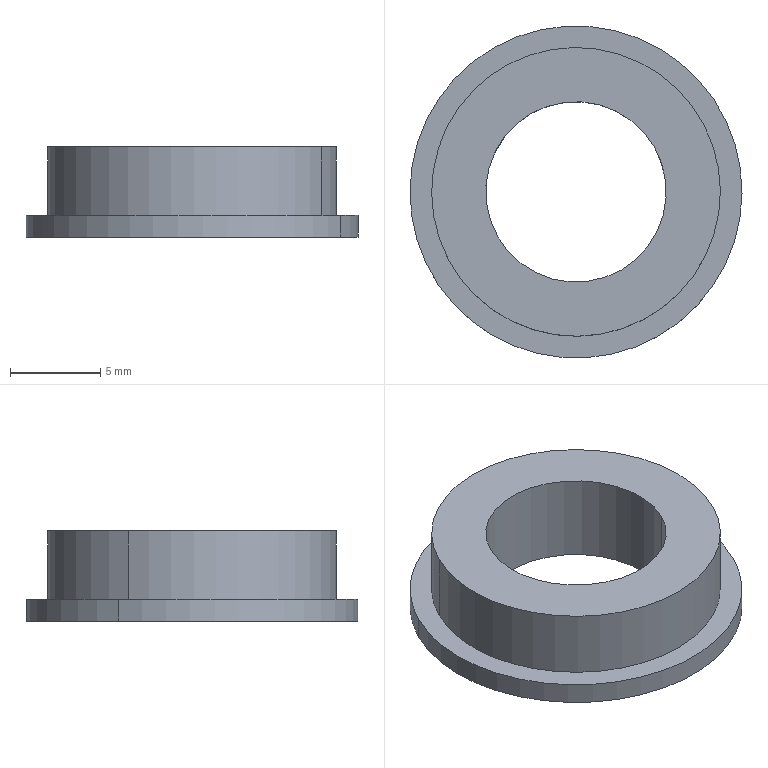Part | NX | features BREP 1 | 1 solid | 9 faces | box 18.4 x 18.4 x 5 mm | volume 690.422 mm3 | cylinder 6 | plane 3 | commonest cylinder face diameters 10 x2 16 x2 18.4 x2
STEP:
#1=CARTESIAN_POINT('',(17.921,165.384,-28.));
#2=VERTEX_POINT('',#1);
#3=CARTESIAN_POINT('',(34.421,157.241,-28.));
#4=VERTEX_POINT('',#3);
#5=CARTESIAN_POINT('',(26.171,161.313,-28.));
#6=DIRECTION('',(0.,0.,1.));
#7=DIRECTION('',(-0.8967,0.4426,0.));
#8=AXIS2_PLACEMENT_3D('',#5,#6,#7);
#9=CIRCLE('',#8,9.2);
#10=EDGE_CURVE('',#2,#4,#9,.T.);
#11=ORIENTED_EDGE('',*,*,#10,.F.);
#12=CARTESIAN_POINT('',(17.921,165.384,-29.2));
#13=VERTEX_POINT('',#12);
#14=CARTESIAN_POINT('',(17.921,165.384,-28.));
#15=DIRECTION('',(0.,0.,-1.));
#16=VECTOR('',#15,1000.);
#17=LINE('',#14,#16);
#18=EDGE_CURVE('',#2,#13,#17,.T.);
#19=ORIENTED_EDGE('',*,*,#18,.T.);
#20=CARTESIAN_POINT('',(34.421,157.241,-29.2));
#21=VERTEX_POINT('',#20);
#22=CARTESIAN_POINT('',(26.171,161.313,-29.2));
#23=DIRECTION('',(0.,0.,1.));
#24=DIRECTION('',(-0.8967,0.4426,0.));
#25=AXIS2_PLACEMENT_3D('',#22,#23,#24);
#26=CIRCLE('',#25,9.2);
#27=EDGE_CURVE('',#13,#21,#26,.T.);
#28=ORIENTED_EDGE('',*,*,#27,.T.);
#29=CARTESIAN_POINT('',(34.421,157.241,-28.));
#30=DIRECTION('',(0.,0.,1.));
#31=VECTOR('',#30,1000.);
#32=LINE('',#29,#31);
#33=EDGE_CURVE('',#21,#4,#32,.T.);
#34=ORIENTED_EDGE('',*,*,#33,.T.);
#35=EDGE_LOOP('',(#11,#19,#28,#34));
#36=FACE_BOUND('',#35,.T.);
#37=CARTESIAN_POINT('',(26.171,161.313,-28.));
#38=DIRECTION('',(0.,0.,-1.));
#39=DIRECTION('',(-0.8967,0.4426,0.));
#40=AXIS2_PLACEMENT_3D('',#37,#38,#39);
#41=CYLINDRICAL_SURFACE('',#40,9.2);
#42=ADVANCED_FACE('',(#36),#41,.T.);
#43=CARTESIAN_POINT('',(30.655,159.1,-24.2));
#44=VERTEX_POINT('',#43);
#45=CARTESIAN_POINT('',(21.687,163.526,-24.2));
#46=VERTEX_POINT('',#45);
#47=CARTESIAN_POINT('',(26.171,161.313,-24.2));
#48=DIRECTION('',(0.,0.,1.));
#49=DIRECTION('',(-0.8967,0.4426,0.));
#50=AXIS2_PLACEMENT_3D('',#47,#48,#49);
#51=CIRCLE('',#50,5.);
#52=EDGE_CURVE('',#44,#46,#51,.T.);
#53=ORIENTED_EDGE('',*,*,#52,.T.);
#54=CARTESIAN_POINT('',(21.687,163.526,-29.2));
#55=VERTEX_POINT('',#54);
#56=CARTESIAN_POINT('',(21.687,163.526,-24.2));
#57=DIRECTION('',(0.,0.,1.));
#58=VECTOR('',#57,1000.);
#59=LINE('',#56,#58);
#60=EDGE_CURVE('',#55,#46,#59,.T.);
#61=ORIENTED_EDGE('',*,*,#60,.F.);
#62=CARTESIAN_POINT('',(30.655,159.1,-29.2));
#63=VERTEX_POINT('',#62);
#64=CARTESIAN_POINT('',(26.171,161.313,-29.2));
#65=DIRECTION('',(0.,0.,1.));
#66=DIRECTION('',(-0.8967,0.4426,0.));
#67=AXIS2_PLACEMENT_3D('',#64,#65,#66);
#68=CIRCLE('',#67,5.);
#69=EDGE_CURVE('',#63,#55,#68,.T.);
#70=ORIENTED_EDGE('',*,*,#69,.F.);
#71=CARTESIAN_POINT('',(30.655,159.1,-24.2));
#72=DIRECTION('',(0.,0.,-1.));
#73=VECTOR('',#72,1000.);
#74=LINE('',#71,#73);
#75=EDGE_CURVE('',#44,#63,#74,.T.);
#76=ORIENTED_EDGE('',*,*,#75,.F.);
#77=EDGE_LOOP('',(#53,#61,#70,#76));
#78=FACE_BOUND('',#77,.T.);
#79=CARTESIAN_POINT('',(26.171,161.313,-24.2));
#80=DIRECTION('',(0.,0.,-1.));
#81=DIRECTION('',(-0.8967,0.4426,0.));
#82=AXIS2_PLACEMENT_3D('',#79,#80,#81);
#83=CYLINDRICAL_SURFACE('',#82,5.);
#84=ADVANCED_FACE('',(#78),#83,.F.);
#85=CARTESIAN_POINT('',(18.997,164.853,-24.2));
#86=VERTEX_POINT('',#85);
#87=CARTESIAN_POINT('',(33.345,157.772,-24.2));
#88=VERTEX_POINT('',#87);
#89=CARTESIAN_POINT('',(26.171,161.313,-24.2));
#90=DIRECTION('',(0.,0.,1.));
#91=DIRECTION('',(-0.8967,0.4426,0.));
#92=AXIS2_PLACEMENT_3D('',#89,#90,#91);
#93=CIRCLE('',#92,8.);
#94=EDGE_CURVE('',#86,#88,#93,.T.);
#95=ORIENTED_EDGE('',*,*,#94,.F.);
#96=CARTESIAN_POINT('',(18.997,164.853,-28.));
#97=VERTEX_POINT('',#96);
#98=CARTESIAN_POINT('',(18.997,164.853,-24.2));
#99=DIRECTION('',(0.,0.,-1.));
#100=VECTOR('',#99,1000.);
#101=LINE('',#98,#100);
#102=EDGE_CURVE('',#86,#97,#101,.T.);
#103=ORIENTED_EDGE('',*,*,#102,.T.);
#104=CARTESIAN_POINT('',(33.345,157.772,-28.));
#105=VERTEX_POINT('',#104);
#106=CARTESIAN_POINT('',(26.171,161.313,-28.));
#107=DIRECTION('',(0.,0.,1.));
#108=DIRECTION('',(-0.8967,0.4426,0.));
#109=AXIS2_PLACEMENT_3D('',#106,#107,#108);
#110=CIRCLE('',#109,8.);
#111=EDGE_CURVE('',#97,#105,#110,.T.);
#112=ORIENTED_EDGE('',*,*,#111,.T.);
#113=CARTESIAN_POINT('',(33.345,157.772,-24.2));
#114=DIRECTION('',(0.,0.,1.));
#115=VECTOR('',#114,1000.);
#116=LINE('',#113,#115);
#117=EDGE_CURVE('',#105,#88,#116,.T.);
#118=ORIENTED_EDGE('',*,*,#117,.T.);
#119=EDGE_LOOP('',(#95,#103,#112,#118));
#120=FACE_BOUND('',#119,.T.);
#121=CARTESIAN_POINT('',(26.171,161.313,-24.2));
#122=DIRECTION('',(0.,0.,-1.));
#123=DIRECTION('',(-0.8967,0.4426,0.));
#124=AXIS2_PLACEMENT_3D('',#121,#122,#123);
#125=CYLINDRICAL_SURFACE('',#124,8.);
#126=ADVANCED_FACE('',(#120),#125,.T.);
#127=CARTESIAN_POINT('',(26.171,161.313,-24.2));
#128=DIRECTION('',(0.,0.,1.));
#129=DIRECTION('',(-0.8967,0.4426,0.));
#130=AXIS2_PLACEMENT_3D('',#127,#128,#129);
#131=CIRCLE('',#130,8.);
#132=EDGE_CURVE('',#88,#86,#131,.T.);
#133=ORIENTED_EDGE('',*,*,#132,.T.);
#134=ORIENTED_EDGE('',*,*,#94,.T.);
#135=EDGE_LOOP('',(#133,#134));
#136=FACE_BOUND('',#135,.T.);
#137=ORIENTED_EDGE('',*,*,#52,.F.);
#138=CARTESIAN_POINT('',(26.171,161.313,-24.2));
#139=DIRECTION('',(0.,0.,1.));
#140=DIRECTION('',(-0.8967,0.4426,0.));
#141=AXIS2_PLACEMENT_3D('',#138,#139,#140);
#142=CIRCLE('',#141,5.);
#143=EDGE_CURVE('',#46,#44,#142,.T.);
#144=ORIENTED_EDGE('',*,*,#143,.F.);
#145=EDGE_LOOP('',(#137,#144));
#146=FACE_BOUND('',#145,.T.);
#147=CARTESIAN_POINT('',(26.171,161.313,-24.2));
#148=DIRECTION('',(0.,0.,1.));
#149=DIRECTION('',(0.8967,-0.4426,0.));
#150=AXIS2_PLACEMENT_3D('',#147,#148,#149);
#151=PLANE('',#150);
#152=ADVANCED_FACE('',(#136,#146),#151,.T.);
#153=ORIENTED_EDGE('',*,*,#69,.T.);
#154=CARTESIAN_POINT('',(26.171,161.313,-29.2));
#155=DIRECTION('',(0.,0.,1.));
#156=DIRECTION('',(-0.8967,0.4426,0.));
#157=AXIS2_PLACEMENT_3D('',#154,#155,#156);
#158=CIRCLE('',#157,5.);
#159=EDGE_CURVE('',#55,#63,#158,.T.);
#160=ORIENTED_EDGE('',*,*,#159,.T.);
#161=EDGE_LOOP('',(#153,#160));
#162=FACE_BOUND('',#161,.T.);
#163=CARTESIAN_POINT('',(26.171,161.313,-29.2));
#164=DIRECTION('',(0.,0.,1.));
#165=DIRECTION('',(-0.8967,0.4426,0.));
#166=AXIS2_PLACEMENT_3D('',#163,#164,#165);
#167=CIRCLE('',#166,9.2);
#168=EDGE_CURVE('',#21,#13,#167,.T.);
#169=ORIENTED_EDGE('',*,*,#168,.F.);
#170=ORIENTED_EDGE('',*,*,#27,.F.);
#171=EDGE_LOOP('',(#169,#170));
#172=FACE_BOUND('',#171,.T.);
#173=CARTESIAN_POINT('',(26.171,161.313,-29.2));
#174=DIRECTION('',(0.,0.,1.));
#175=DIRECTION('',(0.8967,-0.4426,0.));
#176=AXIS2_PLACEMENT_3D('',#173,#174,#175);
#177=PLANE('',#176);
#178=ADVANCED_FACE('',(#162,#172),#177,.F.);
#179=ORIENTED_EDGE('',*,*,#102,.F.);
#180=ORIENTED_EDGE('',*,*,#132,.F.);
#181=ORIENTED_EDGE('',*,*,#117,.F.);
#182=CARTESIAN_POINT('',(26.171,161.313,-28.));
#183=DIRECTION('',(0.,0.,1.));
#184=DIRECTION('',(-0.8967,0.4426,0.));
#185=AXIS2_PLACEMENT_3D('',#182,#183,#184);
#186=CIRCLE('',#185,8.);
#187=EDGE_CURVE('',#105,#97,#186,.T.);
#188=ORIENTED_EDGE('',*,*,#187,.T.);
#189=EDGE_LOOP('',(#179,#180,#181,#188));
#190=FACE_BOUND('',#189,.T.);
#191=CARTESIAN_POINT('',(26.171,161.313,-24.2));
#192=DIRECTION('',(0.,0.,-1.));
#193=DIRECTION('',(-0.8967,0.4426,0.));
#194=AXIS2_PLACEMENT_3D('',#191,#192,#193);
#195=CYLINDRICAL_SURFACE('',#194,8.);
#196=ADVANCED_FACE('',(#190),#195,.T.);
#197=ORIENTED_EDGE('',*,*,#60,.T.);
#198=ORIENTED_EDGE('',*,*,#143,.T.);
#199=ORIENTED_EDGE('',*,*,#75,.T.);
#200=ORIENTED_EDGE('',*,*,#159,.F.);
#201=EDGE_LOOP('',(#197,#198,#199,#200));
#202=FACE_BOUND('',#201,.T.);
#203=CARTESIAN_POINT('',(26.171,161.313,-24.2));
#204=DIRECTION('',(0.,0.,-1.));
#205=DIRECTION('',(-0.8967,0.4426,0.));
#206=AXIS2_PLACEMENT_3D('',#203,#204,#205);
#207=CYLINDRICAL_SURFACE('',#206,5.);
#208=ADVANCED_FACE('',(#202),#207,.F.);
#209=CARTESIAN_POINT('',(26.171,161.313,-28.));
#210=DIRECTION('',(0.,0.,1.));
#211=DIRECTION('',(-0.8967,0.4426,0.));
#212=AXIS2_PLACEMENT_3D('',#209,#210,#211);
#213=CIRCLE('',#212,9.2);
#214=EDGE_CURVE('',#4,#2,#213,.T.);
#215=ORIENTED_EDGE('',*,*,#214,.T.);
#216=ORIENTED_EDGE('',*,*,#10,.T.);
#217=EDGE_LOOP('',(#215,#216));
#218=FACE_BOUND('',#217,.T.);
#219=ORIENTED_EDGE('',*,*,#187,.F.);
#220=ORIENTED_EDGE('',*,*,#111,.F.);
#221=EDGE_LOOP('',(#219,#220));
#222=FACE_BOUND('',#221,.T.);
#223=CARTESIAN_POINT('',(26.171,161.313,-28.));
#224=DIRECTION('',(0.,0.,1.));
#225=DIRECTION('',(0.8967,-0.4426,0.));
#226=AXIS2_PLACEMENT_3D('',#223,#224,#225);
#227=PLANE('',#226);
#228=ADVANCED_FACE('',(#218,#222),#227,.T.);
#229=ORIENTED_EDGE('',*,*,#18,.F.);
#230=ORIENTED_EDGE('',*,*,#214,.F.);
#231=ORIENTED_EDGE('',*,*,#33,.F.);
#232=ORIENTED_EDGE('',*,*,#168,.T.);
#233=EDGE_LOOP('',(#229,#230,#231,#232));
#234=FACE_BOUND('',#233,.T.);
#235=CARTESIAN_POINT('',(26.171,161.313,-28.));
#236=DIRECTION('',(0.,0.,-1.));
#237=DIRECTION('',(-0.8967,0.4426,0.));
#238=AXIS2_PLACEMENT_3D('',#235,#236,#237);
#239=CYLINDRICAL_SURFACE('',#238,9.2);
#240=ADVANCED_FACE('',(#234),#239,.T.);
#241=CLOSED_SHELL('',(#42,#84,#126,#152,#178,#196,#208,#228,#240));
#242=MANIFOLD_SOLID_BREP('',#241);
#243=(LENGTH_UNIT()NAMED_UNIT(*)SI_UNIT(.MILLI.,.METRE.));
#244=UNCERTAINTY_MEASURE_WITH_UNIT(LENGTH_MEASURE(0.00001),#243,'','');
#245=(NAMED_UNIT(*)PLANE_ANGLE_UNIT()SI_UNIT($,.RADIAN.));
#246=(NAMED_UNIT(*)SI_UNIT($,.STERADIAN.)SOLID_ANGLE_UNIT());
#247=(GEOMETRIC_REPRESENTATION_CONTEXT(3)GLOBAL_UNCERTAINTY_ASSIGNED_CONTEXT((#244))GLOBAL_UNIT_ASSIGNED_CONTEXT((#243,#245,#246))REPRESENTATION_CONTEXT('',''));
#248=ADVANCED_BREP_SHAPE_REPRESENTATION('',(#242),#247);